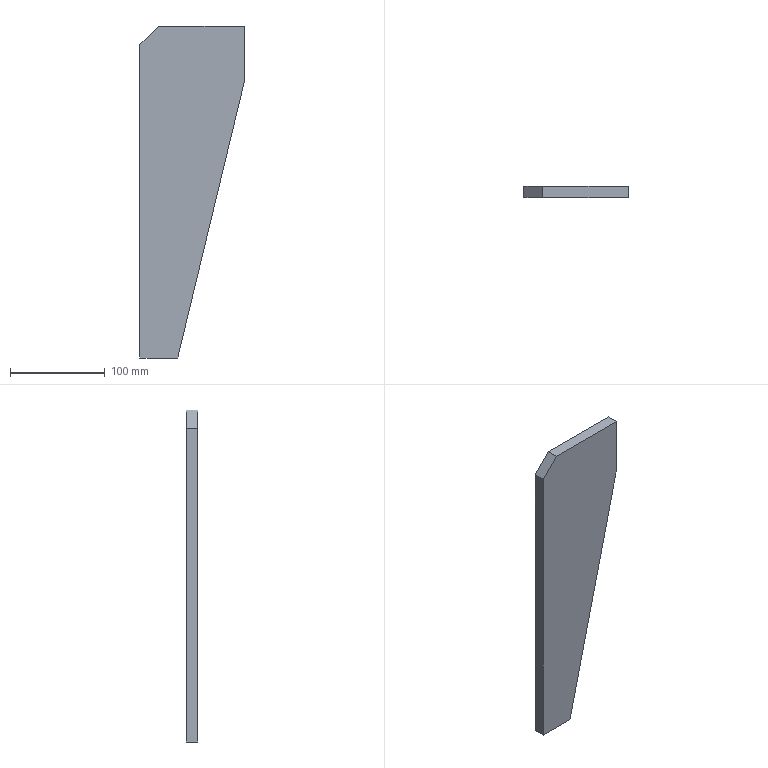Part | SolidWorks | features Chamfer 1, Extrusion 1 | 1 solid | 8 faces | box 110 x 12 x 350 mm | volume 337800 mm3 | plane 8
STEP:
#1=CARTESIAN_POINT('',(0.,6.,0.));
#2=VERTEX_POINT('',#1);
#3=CARTESIAN_POINT('',(90.,6.,0.));
#4=VERTEX_POINT('',#3);
#5=CARTESIAN_POINT('',(-20.,6.,0.));
#6=DIRECTION('',(1.,0.,0.));
#7=VECTOR('',#6,1000.);
#8=LINE('',#5,#7);
#9=EDGE_CURVE('',#2,#4,#8,.T.);
#10=ORIENTED_EDGE('',*,*,#9,.F.);
#11=CARTESIAN_POINT('',(0.,-6.,0.));
#12=VERTEX_POINT('',#11);
#13=CARTESIAN_POINT('',(0.,6.,0.));
#14=DIRECTION('',(0.,-1.,0.));
#15=VECTOR('',#14,1000.);
#16=LINE('',#13,#15);
#17=EDGE_CURVE('',#2,#12,#16,.T.);
#18=ORIENTED_EDGE('',*,*,#17,.T.);
#19=CARTESIAN_POINT('',(90.,-6.,0.));
#20=VERTEX_POINT('',#19);
#21=CARTESIAN_POINT('',(90.,-6.,0.));
#22=DIRECTION('',(1.,0.,0.));
#23=VECTOR('',#22,1000.);
#24=LINE('',#21,#23);
#25=EDGE_CURVE('',#12,#20,#24,.T.);
#26=ORIENTED_EDGE('',*,*,#25,.T.);
#27=CARTESIAN_POINT('',(90.,6.,0.));
#28=DIRECTION('',(0.,-1.,0.));
#29=VECTOR('',#28,1000.);
#30=LINE('',#27,#29);
#31=EDGE_CURVE('',#4,#20,#30,.T.);
#32=ORIENTED_EDGE('',*,*,#31,.F.);
#33=EDGE_LOOP('',(#10,#18,#26,#32));
#34=FACE_OUTER_BOUND('',#33,.T.);
#35=CARTESIAN_POINT('',(90.,6.,0.));
#36=DIRECTION('',(0.,0.,-1.));
#37=DIRECTION('',(-1.,0.,0.));
#38=AXIS2_PLACEMENT_3D('',#35,#36,#37);
#39=PLANE('',#38);
#40=ADVANCED_FACE('',(#34),#39,.F.);
#41=CARTESIAN_POINT('',(90.,-6.,-60.));
#42=VERTEX_POINT('',#41);
#43=CARTESIAN_POINT('',(90.,-6.,-60.));
#44=DIRECTION('',(0.,0.,-1.));
#45=VECTOR('',#44,1000.);
#46=LINE('',#43,#45);
#47=EDGE_CURVE('',#20,#42,#46,.T.);
#48=ORIENTED_EDGE('',*,*,#47,.T.);
#49=CARTESIAN_POINT('',(90.,6.,-60.));
#50=VERTEX_POINT('',#49);
#51=CARTESIAN_POINT('',(90.,6.,-60.));
#52=DIRECTION('',(0.,-1.,0.));
#53=VECTOR('',#52,1000.);
#54=LINE('',#51,#53);
#55=EDGE_CURVE('',#50,#42,#54,.T.);
#56=ORIENTED_EDGE('',*,*,#55,.F.);
#57=CARTESIAN_POINT('',(90.,6.,-60.));
#58=DIRECTION('',(0.,0.,-1.));
#59=VECTOR('',#58,1000.);
#60=LINE('',#57,#59);
#61=EDGE_CURVE('',#4,#50,#60,.T.);
#62=ORIENTED_EDGE('',*,*,#61,.F.);
#63=ORIENTED_EDGE('',*,*,#31,.T.);
#64=EDGE_LOOP('',(#48,#56,#62,#63));
#65=FACE_OUTER_BOUND('',#64,.T.);
#66=CARTESIAN_POINT('',(90.,6.,-60.));
#67=DIRECTION('',(-1.,0.,0.));
#68=DIRECTION('',(0.,0.,1.));
#69=AXIS2_PLACEMENT_3D('',#66,#67,#68);
#70=PLANE('',#69);
#71=ADVANCED_FACE('',(#65),#70,.F.);
#72=CARTESIAN_POINT('',(20.,-6.,-350.));
#73=VERTEX_POINT('',#72);
#74=CARTESIAN_POINT('',(20.,-6.,-350.));
#75=DIRECTION('',(-0.2346,0.,-0.9721));
#76=VECTOR('',#75,1000.);
#77=LINE('',#74,#76);
#78=EDGE_CURVE('',#42,#73,#77,.T.);
#79=ORIENTED_EDGE('',*,*,#78,.T.);
#80=CARTESIAN_POINT('',(20.,6.,-350.));
#81=VERTEX_POINT('',#80);
#82=CARTESIAN_POINT('',(20.,6.,-350.));
#83=DIRECTION('',(0.,-1.,0.));
#84=VECTOR('',#83,1000.);
#85=LINE('',#82,#84);
#86=EDGE_CURVE('',#81,#73,#85,.T.);
#87=ORIENTED_EDGE('',*,*,#86,.F.);
#88=CARTESIAN_POINT('',(20.,6.,-350.));
#89=DIRECTION('',(-0.2346,0.,-0.9721));
#90=VECTOR('',#89,1000.);
#91=LINE('',#88,#90);
#92=EDGE_CURVE('',#50,#81,#91,.T.);
#93=ORIENTED_EDGE('',*,*,#92,.F.);
#94=ORIENTED_EDGE('',*,*,#55,.T.);
#95=EDGE_LOOP('',(#79,#87,#93,#94));
#96=FACE_OUTER_BOUND('',#95,.T.);
#97=CARTESIAN_POINT('',(20.,6.,-350.));
#98=DIRECTION('',(-0.9721,0.,0.2346));
#99=DIRECTION('',(0.2346,0.,0.9721));
#100=AXIS2_PLACEMENT_3D('',#97,#98,#99);
#101=PLANE('',#100);
#102=ADVANCED_FACE('',(#96),#101,.F.);
#103=CARTESIAN_POINT('',(-20.,-6.,-350.));
#104=VERTEX_POINT('',#103);
#105=CARTESIAN_POINT('',(-20.,-6.,-350.));
#106=DIRECTION('',(-1.,0.,0.));
#107=VECTOR('',#106,1000.);
#108=LINE('',#105,#107);
#109=EDGE_CURVE('',#73,#104,#108,.T.);
#110=ORIENTED_EDGE('',*,*,#109,.T.);
#111=CARTESIAN_POINT('',(-20.,6.,-350.));
#112=VERTEX_POINT('',#111);
#113=CARTESIAN_POINT('',(-20.,6.,-350.));
#114=DIRECTION('',(0.,-1.,0.));
#115=VECTOR('',#114,1000.);
#116=LINE('',#113,#115);
#117=EDGE_CURVE('',#112,#104,#116,.T.);
#118=ORIENTED_EDGE('',*,*,#117,.F.);
#119=CARTESIAN_POINT('',(-20.,6.,-350.));
#120=DIRECTION('',(-1.,0.,0.));
#121=VECTOR('',#120,1000.);
#122=LINE('',#119,#121);
#123=EDGE_CURVE('',#81,#112,#122,.T.);
#124=ORIENTED_EDGE('',*,*,#123,.F.);
#125=ORIENTED_EDGE('',*,*,#86,.T.);
#126=EDGE_LOOP('',(#110,#118,#124,#125));
#127=FACE_OUTER_BOUND('',#126,.T.);
#128=CARTESIAN_POINT('',(-20.,6.,-350.));
#129=DIRECTION('',(0.,0.,1.));
#130=DIRECTION('',(1.,0.,0.));
#131=AXIS2_PLACEMENT_3D('',#128,#129,#130);
#132=PLANE('',#131);
#133=ADVANCED_FACE('',(#127),#132,.F.);
#134=CARTESIAN_POINT('',(-20.,-6.,-20.));
#135=VERTEX_POINT('',#134);
#136=CARTESIAN_POINT('',(-20.,-6.,-20.));
#137=DIRECTION('',(0.,0.,1.));
#138=VECTOR('',#137,1000.);
#139=LINE('',#136,#138);
#140=EDGE_CURVE('',#104,#135,#139,.T.);
#141=ORIENTED_EDGE('',*,*,#140,.T.);
#142=CARTESIAN_POINT('',(-20.,6.,-20.));
#143=VERTEX_POINT('',#142);
#144=CARTESIAN_POINT('',(-20.,6.,-20.));
#145=DIRECTION('',(0.,1.,0.));
#146=VECTOR('',#145,1000.);
#147=LINE('',#144,#146);
#148=EDGE_CURVE('',#135,#143,#147,.T.);
#149=ORIENTED_EDGE('',*,*,#148,.T.);
#150=CARTESIAN_POINT('',(-20.,6.,-20.));
#151=DIRECTION('',(0.,0.,1.));
#152=VECTOR('',#151,1000.);
#153=LINE('',#150,#152);
#154=EDGE_CURVE('',#112,#143,#153,.T.);
#155=ORIENTED_EDGE('',*,*,#154,.F.);
#156=ORIENTED_EDGE('',*,*,#117,.T.);
#157=EDGE_LOOP('',(#141,#149,#155,#156));
#158=FACE_OUTER_BOUND('',#157,.T.);
#159=CARTESIAN_POINT('',(-20.,6.,-20.));
#160=DIRECTION('',(1.,0.,0.));
#161=DIRECTION('',(0.,0.,-1.));
#162=AXIS2_PLACEMENT_3D('',#159,#160,#161);
#163=PLANE('',#162);
#164=ADVANCED_FACE('',(#158),#163,.F.);
#165=ORIENTED_EDGE('',*,*,#154,.T.);
#166=CARTESIAN_POINT('',(0.,6.,0.));
#167=DIRECTION('',(0.7071,0.,0.7071));
#168=VECTOR('',#167,1000.);
#169=LINE('',#166,#168);
#170=EDGE_CURVE('',#143,#2,#169,.T.);
#171=ORIENTED_EDGE('',*,*,#170,.T.);
#172=ORIENTED_EDGE('',*,*,#9,.T.);
#173=ORIENTED_EDGE('',*,*,#61,.T.);
#174=ORIENTED_EDGE('',*,*,#92,.T.);
#175=ORIENTED_EDGE('',*,*,#123,.T.);
#176=EDGE_LOOP('',(#165,#171,#172,#173,#174,#175));
#177=FACE_OUTER_BOUND('',#176,.T.);
#178=CARTESIAN_POINT('',(0.,6.,0.));
#179=DIRECTION('',(0.,-1.,0.));
#180=DIRECTION('',(0.,0.,-1.));
#181=AXIS2_PLACEMENT_3D('',#178,#179,#180);
#182=PLANE('',#181);
#183=ADVANCED_FACE('',(#177),#182,.F.);
#184=ORIENTED_EDGE('',*,*,#25,.F.);
#185=CARTESIAN_POINT('',(0.,-6.,0.));
#186=DIRECTION('',(-0.7071,0.,-0.7071));
#187=VECTOR('',#186,1000.);
#188=LINE('',#185,#187);
#189=EDGE_CURVE('',#12,#135,#188,.T.);
#190=ORIENTED_EDGE('',*,*,#189,.T.);
#191=ORIENTED_EDGE('',*,*,#140,.F.);
#192=ORIENTED_EDGE('',*,*,#109,.F.);
#193=ORIENTED_EDGE('',*,*,#78,.F.);
#194=ORIENTED_EDGE('',*,*,#47,.F.);
#195=EDGE_LOOP('',(#184,#190,#191,#192,#193,#194));
#196=FACE_OUTER_BOUND('',#195,.T.);
#197=CARTESIAN_POINT('',(0.,-6.,0.));
#198=DIRECTION('',(0.,-1.,0.));
#199=DIRECTION('',(0.,0.,-1.));
#200=AXIS2_PLACEMENT_3D('',#197,#198,#199);
#201=PLANE('',#200);
#202=ADVANCED_FACE('',(#196),#201,.T.);
#203=ORIENTED_EDGE('',*,*,#170,.F.);
#204=ORIENTED_EDGE('',*,*,#148,.F.);
#205=ORIENTED_EDGE('',*,*,#189,.F.);
#206=ORIENTED_EDGE('',*,*,#17,.F.);
#207=EDGE_LOOP('',(#203,#204,#205,#206));
#208=FACE_OUTER_BOUND('',#207,.T.);
#209=CARTESIAN_POINT('',(0.,6.,0.));
#210=DIRECTION('',(0.7071,0.,-0.7071));
#211=DIRECTION('',(0.,-1.,0.));
#212=AXIS2_PLACEMENT_3D('',#209,#210,#211);
#213=PLANE('',#212);
#214=ADVANCED_FACE('',(#208),#213,.F.);
#215=CLOSED_SHELL('',(#40,#71,#102,#133,#164,#183,#202,#214));
#216=MANIFOLD_SOLID_BREP('',#215);
#217=CARTESIAN_POINT('',(0.,0.,0.));
#218=DIRECTION('',(0.,0.,1.));
#219=DIRECTION('',(1.,0.,0.));
#220=AXIS2_PLACEMENT_3D('',#217,#218,#219);
#221=(LENGTH_UNIT()NAMED_UNIT(*)SI_UNIT(.MILLI.,.METRE.));
#222=UNCERTAINTY_MEASURE_WITH_UNIT(LENGTH_MEASURE(0.00001),#221,'','');
#223=(NAMED_UNIT(*)PLANE_ANGLE_UNIT()SI_UNIT($,.RADIAN.));
#224=(NAMED_UNIT(*)SI_UNIT($,.STERADIAN.)SOLID_ANGLE_UNIT());
#225=(GEOMETRIC_REPRESENTATION_CONTEXT(3)GLOBAL_UNCERTAINTY_ASSIGNED_CONTEXT((#222))GLOBAL_UNIT_ASSIGNED_CONTEXT((#221,#223,#224))REPRESENTATION_CONTEXT('',''));
#226=ADVANCED_BREP_SHAPE_REPRESENTATION('',(#216,#220),#225);